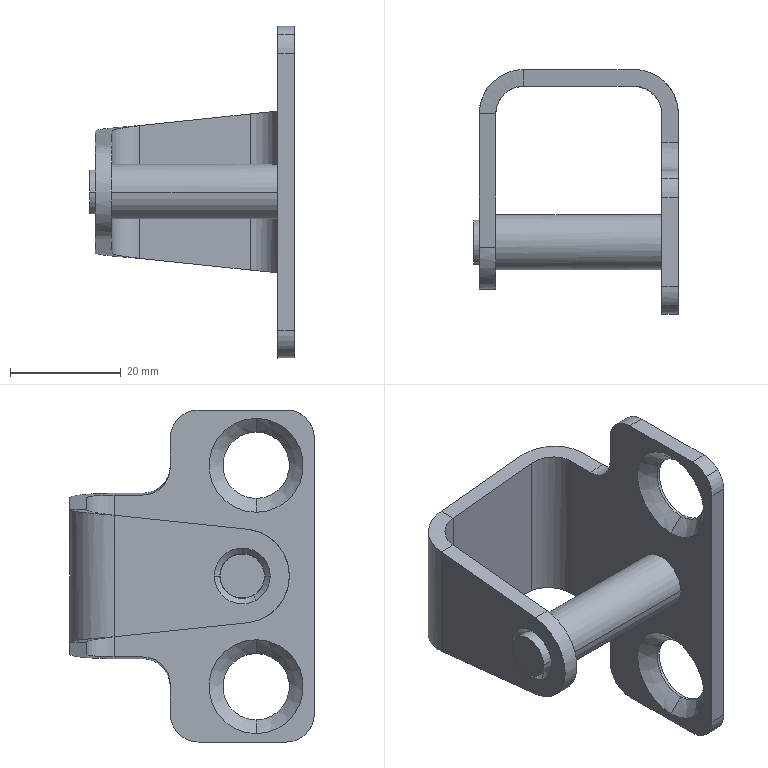Part | NX | features BREP 2 | 2 solids | 62 faces | box 37 x 44.176 x 60 mm | volume 11849 mm3 | cylinder 27 | plane 19 | cone 14 | spline 2 | commonest cylinder face diameters 10 x16 12 x4 8 x2 8.1 x2 16 x2 17 x1